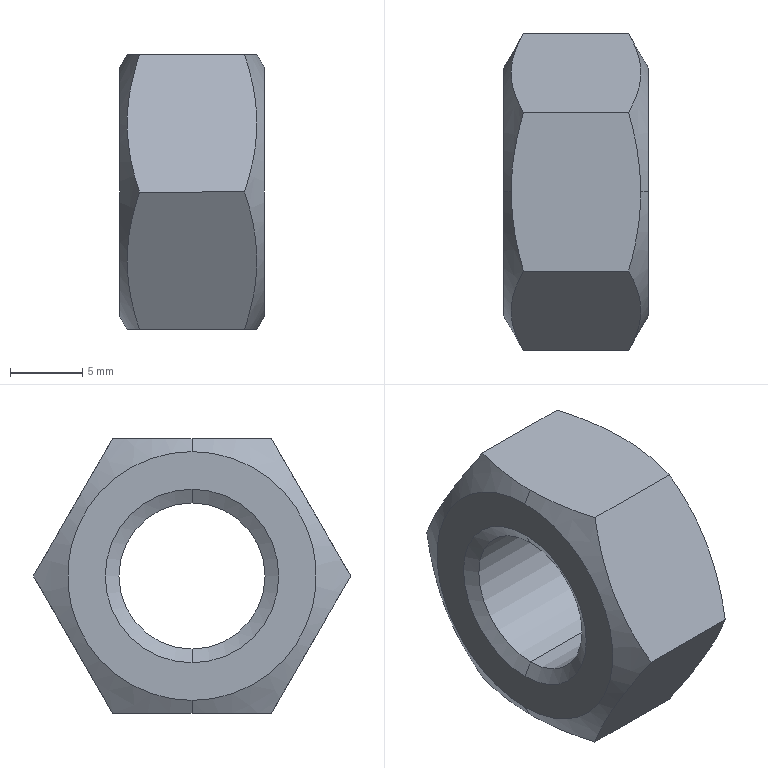Part | STEP file | DIN 934 - M12 x 1,75 | 1 solid | 18 faces | box 10 x 21.939 x 19 mm | volume 2235 mm3 | cone 8 | plane 8 | cylinder 2 | commonest cylinder face diameters 10.106 x2